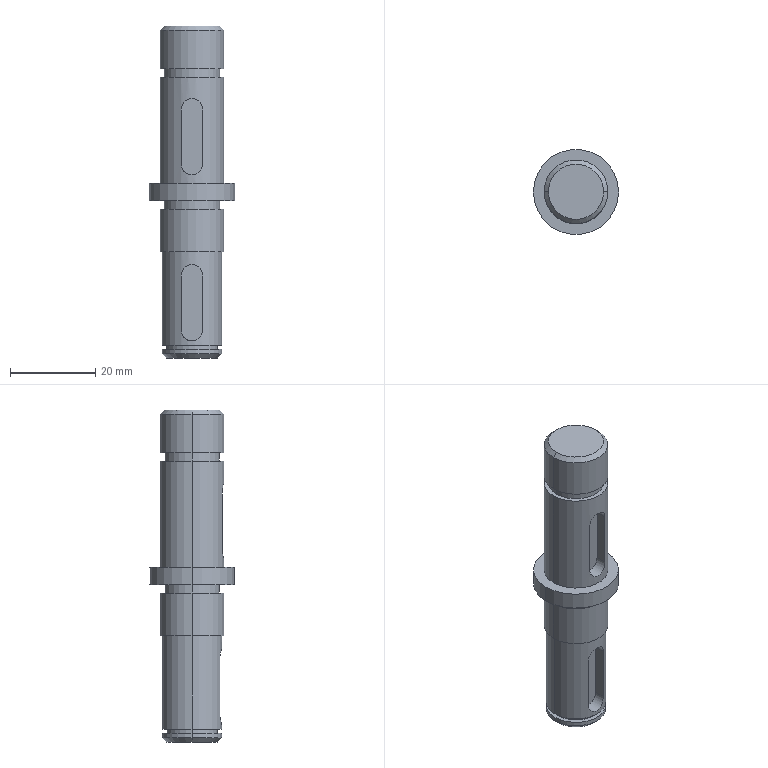Part | SolidWorks | features ICE 10, Chamfer 1, Extrusion 1 | 1 solid | 44 faces | box 20 x 20 x 78 mm | volume 13019 mm3 | cylinder 24 | plane 16 | cone 4 | commonest cylinder face diameters 5 x6 15 x6 13 x4 14 x4 12 x2 20 x2
STEP:
#1=CARTESIAN_POINT('',(0.,-7.5,61.));
#2=VERTEX_POINT('',#1);
#3=CARTESIAN_POINT('',(2.5,-7.071,58.5));
#4=VERTEX_POINT('',#3);
#5=CARTESIAN_POINT('',(0.,-7.5,61.));
#6=CARTESIAN_POINT('',(0.1643,-7.5,61.));
#7=CARTESIAN_POINT('',(0.3311,-7.494,60.983));
#8=CARTESIAN_POINT('',(0.6524,-7.473,60.919));
#9=CARTESIAN_POINT('',(0.8088,-7.458,60.871));
#10=CARTESIAN_POINT('',(1.113,-7.419,60.745));
#11=CARTESIAN_POINT('',(1.257,-7.395,60.667));
#12=CARTESIAN_POINT('',(1.526,-7.344,60.487));
#13=CARTESIAN_POINT('',(1.653,-7.316,60.382));
#14=CARTESIAN_POINT('',(1.883,-7.261,60.152));
#15=CARTESIAN_POINT('',(1.986,-7.233,60.027));
#16=CARTESIAN_POINT('',(2.167,-7.181,59.758));
#17=CARTESIAN_POINT('',(2.245,-7.156,59.612));
#18=CARTESIAN_POINT('',(2.37,-7.116,59.311));
#19=CARTESIAN_POINT('',(2.418,-7.1,59.156));
#20=CARTESIAN_POINT('',(2.483,-7.077,58.832));
#21=CARTESIAN_POINT('',(2.5,-7.071,58.666));
#22=CARTESIAN_POINT('',(2.5,-7.071,58.5));
#23=B_SPLINE_CURVE_WITH_KNOTS('',3,(#5,#6,#7,#8,#9,#10,#11,#12,#13,#14,#15,#16,#17,#18,#19,#20,#21,#22),.UNSPECIFIED.,.F.,.F.,(4,2,2,2,2,2,2,2,4),(0.003937,0.004429,0.004921,0.005412,0.005904,0.006395,0.006887,0.007378,0.00787),.UNSPECIFIED.);
#24=EDGE_CURVE('',#2,#4,#23,.T.);
#25=ORIENTED_EDGE('',*,*,#24,.F.);
#26=CARTESIAN_POINT('',(0.,-4.5,61.));
#27=VERTEX_POINT('',#26);
#28=CARTESIAN_POINT('',(0.,-14.5,61.));
#29=DIRECTION('',(0.,1.,0.));
#30=VECTOR('',#29,1000.);
#31=LINE('',#28,#30);
#32=EDGE_CURVE('',#2,#27,#31,.T.);
#33=ORIENTED_EDGE('',*,*,#32,.T.);
#34=CARTESIAN_POINT('',(2.5,-4.5,58.5));
#35=VERTEX_POINT('',#34);
#36=CARTESIAN_POINT('',(0.,-4.5,58.5));
#37=DIRECTION('',(0.,1.,0.));
#38=DIRECTION('',(0.,0.,1.));
#39=AXIS2_PLACEMENT_3D('',#36,#37,#38);
#40=CIRCLE('',#39,2.5);
#41=EDGE_CURVE('',#27,#35,#40,.T.);
#42=ORIENTED_EDGE('',*,*,#41,.T.);
#43=CARTESIAN_POINT('',(2.5,-14.5,58.5));
#44=DIRECTION('',(0.,1.,0.));
#45=VECTOR('',#44,1000.);
#46=LINE('',#43,#45);
#47=EDGE_CURVE('',#4,#35,#46,.T.);
#48=ORIENTED_EDGE('',*,*,#47,.F.);
#49=EDGE_LOOP('',(#25,#33,#42,#48));
#50=FACE_OUTER_BOUND('',#49,.T.);
#51=CARTESIAN_POINT('',(0.,-14.5,58.5));
#52=DIRECTION('',(0.,1.,0.));
#53=DIRECTION('',(0.,0.,1.));
#54=AXIS2_PLACEMENT_3D('',#51,#52,#53);
#55=CYLINDRICAL_SURFACE('',#54,2.5);
#56=ADVANCED_FACE('',(#50),#55,.F.);
#57=CARTESIAN_POINT('',(0.,-7.,22.));
#58=VERTEX_POINT('',#57);
#59=CARTESIAN_POINT('',(2.5,-6.538,19.5));
#60=VERTEX_POINT('',#59);
#61=CARTESIAN_POINT('',(0.,-7.,22.));
#62=CARTESIAN_POINT('',(0.1645,-7.,22.));
#63=CARTESIAN_POINT('',(0.3315,-6.994,21.983));
#64=CARTESIAN_POINT('',(0.653,-6.971,21.919));
#65=CARTESIAN_POINT('',(0.8095,-6.955,21.871));
#66=CARTESIAN_POINT('',(1.114,-6.913,21.744));
#67=CARTESIAN_POINT('',(1.257,-6.888,21.667));
#68=CARTESIAN_POINT('',(1.527,-6.833,21.486));
#69=CARTESIAN_POINT('',(1.654,-6.803,21.382));
#70=CARTESIAN_POINT('',(1.883,-6.743,21.152));
#71=CARTESIAN_POINT('',(1.986,-6.713,21.028));
#72=CARTESIAN_POINT('',(2.166,-6.657,20.758));
#73=CARTESIAN_POINT('',(2.245,-6.631,20.612));
#74=CARTESIAN_POINT('',(2.37,-6.587,20.312));
#75=CARTESIAN_POINT('',(2.418,-6.569,20.156));
#76=CARTESIAN_POINT('',(2.483,-6.545,19.833));
#77=CARTESIAN_POINT('',(2.5,-6.538,19.667));
#78=CARTESIAN_POINT('',(2.5,-6.538,19.5));
#79=B_SPLINE_CURVE_WITH_KNOTS('',3,(#61,#62,#63,#64,#65,#66,#67,#68,#69,#70,#71,#72,#73,#74,#75,#76,#77,#78),.UNSPECIFIED.,.F.,.F.,(4,2,2,2,2,2,2,2,4),(0.003942,0.004434,0.004926,0.005418,0.00591,0.006402,0.006894,0.007386,0.007878),.UNSPECIFIED.);
#80=EDGE_CURVE('',#58,#60,#79,.T.);
#81=ORIENTED_EDGE('',*,*,#80,.F.);
#82=CARTESIAN_POINT('',(0.,-4.,22.));
#83=VERTEX_POINT('',#82);
#84=CARTESIAN_POINT('',(0.,-14.,22.));
#85=DIRECTION('',(0.,1.,0.));
#86=VECTOR('',#85,1000.);
#87=LINE('',#84,#86);
#88=EDGE_CURVE('',#58,#83,#87,.T.);
#89=ORIENTED_EDGE('',*,*,#88,.T.);
#90=CARTESIAN_POINT('',(2.5,-4.,19.5));
#91=VERTEX_POINT('',#90);
#92=CARTESIAN_POINT('',(0.,-4.,19.5));
#93=DIRECTION('',(0.,1.,0.));
#94=DIRECTION('',(0.,0.,1.));
#95=AXIS2_PLACEMENT_3D('',#92,#93,#94);
#96=CIRCLE('',#95,2.5);
#97=EDGE_CURVE('',#83,#91,#96,.T.);
#98=ORIENTED_EDGE('',*,*,#97,.T.);
#99=CARTESIAN_POINT('',(2.5,-14.,19.5));
#100=DIRECTION('',(0.,1.,0.));
#101=VECTOR('',#100,1000.);
#102=LINE('',#99,#101);
#103=EDGE_CURVE('',#60,#91,#102,.T.);
#104=ORIENTED_EDGE('',*,*,#103,.F.);
#105=EDGE_LOOP('',(#81,#89,#98,#104));
#106=FACE_OUTER_BOUND('',#105,.T.);
#107=CARTESIAN_POINT('',(0.,-14.,19.5));
#108=DIRECTION('',(0.,1.,0.));
#109=DIRECTION('',(0.,0.,1.));
#110=AXIS2_PLACEMENT_3D('',#107,#108,#109);
#111=CYLINDRICAL_SURFACE('',#110,2.5);
#112=ADVANCED_FACE('',(#106),#111,.F.);
#113=CARTESIAN_POINT('',(6.5,0.,78.));
#114=VERTEX_POINT('',#113);
#115=CARTESIAN_POINT('',(-6.5,0.,78.));
#116=VERTEX_POINT('',#115);
#117=CARTESIAN_POINT('',(0.,0.,78.));
#118=DIRECTION('',(0.,0.,1.));
#119=DIRECTION('',(1.,0.,0.));
#120=AXIS2_PLACEMENT_3D('',#117,#118,#119);
#121=CIRCLE('',#120,6.5);
#122=EDGE_CURVE('',#114,#116,#121,.T.);
#123=ORIENTED_EDGE('',*,*,#122,.F.);
#124=CARTESIAN_POINT('',(7.5,0.,77.));
#125=VERTEX_POINT('',#124);
#126=CARTESIAN_POINT('',(6.5,0.,78.));
#127=DIRECTION('',(0.7071,0.,-0.7071));
#128=VECTOR('',#127,1000.);
#129=LINE('',#126,#128);
#130=EDGE_CURVE('',#114,#125,#129,.T.);
#131=ORIENTED_EDGE('',*,*,#130,.T.);
#132=CARTESIAN_POINT('',(-7.5,0.,77.));
#133=VERTEX_POINT('',#132);
#134=CARTESIAN_POINT('',(0.,0.,77.));
#135=DIRECTION('',(0.,0.,-1.));
#136=DIRECTION('',(1.,0.,0.));
#137=AXIS2_PLACEMENT_3D('',#134,#135,#136);
#138=CIRCLE('',#137,7.5);
#139=EDGE_CURVE('',#133,#125,#138,.T.);
#140=ORIENTED_EDGE('',*,*,#139,.F.);
#141=CARTESIAN_POINT('',(-6.5,0.,78.));
#142=DIRECTION('',(-0.7071,0.,-0.7071));
#143=VECTOR('',#142,1000.);
#144=LINE('',#141,#143);
#145=EDGE_CURVE('',#116,#133,#144,.T.);
#146=ORIENTED_EDGE('',*,*,#145,.F.);
#147=EDGE_LOOP('',(#123,#131,#140,#146));
#148=FACE_OUTER_BOUND('',#147,.T.);
#149=CARTESIAN_POINT('',(0.,0.,78.));
#150=DIRECTION('',(0.,0.,-1.));
#151=DIRECTION('',(-1.,0.,0.));
#152=AXIS2_PLACEMENT_3D('',#149,#150,#151);
#153=CONICAL_SURFACE('',#152,6.5,0.7854);
#154=ADVANCED_FACE('',(#148),#153,.T.);
#155=CARTESIAN_POINT('',(-6.,0.,0.));
#156=VERTEX_POINT('',#155);
#157=CARTESIAN_POINT('',(6.,0.,0.));
#158=VERTEX_POINT('',#157);
#159=CARTESIAN_POINT('',(0.,0.,0.));
#160=DIRECTION('',(0.,0.,-1.));
#161=DIRECTION('',(1.,0.,0.));
#162=AXIS2_PLACEMENT_3D('',#159,#160,#161);
#163=CIRCLE('',#162,6.);
#164=EDGE_CURVE('',#156,#158,#163,.T.);
#165=ORIENTED_EDGE('',*,*,#164,.F.);
#166=CARTESIAN_POINT('',(-7.,0.,1.));
#167=VERTEX_POINT('',#166);
#168=CARTESIAN_POINT('',(-7.,0.,1.));
#169=DIRECTION('',(-0.7071,0.,0.7071));
#170=VECTOR('',#169,1000.);
#171=LINE('',#168,#170);
#172=EDGE_CURVE('',#156,#167,#171,.T.);
#173=ORIENTED_EDGE('',*,*,#172,.T.);
#174=CARTESIAN_POINT('',(7.,0.,1.));
#175=VERTEX_POINT('',#174);
#176=CARTESIAN_POINT('',(0.,0.,1.));
#177=DIRECTION('',(0.,0.,1.));
#178=DIRECTION('',(1.,0.,0.));
#179=AXIS2_PLACEMENT_3D('',#176,#177,#178);
#180=CIRCLE('',#179,7.);
#181=EDGE_CURVE('',#175,#167,#180,.T.);
#182=ORIENTED_EDGE('',*,*,#181,.F.);
#183=CARTESIAN_POINT('',(7.,0.,1.));
#184=DIRECTION('',(0.7071,0.,0.7071));
#185=VECTOR('',#184,1000.);
#186=LINE('',#183,#185);
#187=EDGE_CURVE('',#158,#175,#186,.T.);
#188=ORIENTED_EDGE('',*,*,#187,.F.);
#189=EDGE_LOOP('',(#165,#173,#182,#188));
#190=FACE_OUTER_BOUND('',#189,.T.);
#191=CARTESIAN_POINT('',(0.,0.,1.));
#192=DIRECTION('',(0.,0.,1.));
#193=DIRECTION('',(1.,0.,0.));
#194=AXIS2_PLACEMENT_3D('',#191,#192,#193);
#195=CONICAL_SURFACE('',#194,7.,0.7854);
#196=ADVANCED_FACE('',(#190),#195,.T.);
#197=ORIENTED_EDGE('',*,*,#139,.T.);
#198=CARTESIAN_POINT('',(7.5,0.,68.));
#199=VERTEX_POINT('',#198);
#200=CARTESIAN_POINT('',(7.5,0.,78.));
#201=DIRECTION('',(0.,0.,-1.));
#202=VECTOR('',#201,1000.);
#203=LINE('',#200,#202);
#204=EDGE_CURVE('',#125,#199,#203,.T.);
#205=ORIENTED_EDGE('',*,*,#204,.T.);
#206=CARTESIAN_POINT('',(-7.5,0.,68.));
#207=VERTEX_POINT('',#206);
#208=CARTESIAN_POINT('',(0.,0.,68.));
#209=DIRECTION('',(0.,0.,1.));
#210=DIRECTION('',(1.,0.,0.));
#211=AXIS2_PLACEMENT_3D('',#208,#209,#210);
#212=CIRCLE('',#211,7.5);
#213=EDGE_CURVE('',#199,#207,#212,.T.);
#214=ORIENTED_EDGE('',*,*,#213,.T.);
#215=CARTESIAN_POINT('',(-7.5,0.,78.));
#216=DIRECTION('',(0.,0.,-1.));
#217=VECTOR('',#216,1000.);
#218=LINE('',#215,#217);
#219=EDGE_CURVE('',#133,#207,#218,.T.);
#220=ORIENTED_EDGE('',*,*,#219,.F.);
#221=EDGE_LOOP('',(#197,#205,#214,#220));
#222=FACE_OUTER_BOUND('',#221,.T.);
#223=CARTESIAN_POINT('',(0.,0.,78.));
#224=DIRECTION('',(0.,0.,-1.));
#225=DIRECTION('',(-1.,0.,0.));
#226=AXIS2_PLACEMENT_3D('',#223,#224,#225);
#227=CYLINDRICAL_SURFACE('',#226,7.5);
#228=ADVANCED_FACE('',(#222),#227,.T.);
#229=CARTESIAN_POINT('',(6.5,0.,68.));
#230=VERTEX_POINT('',#229);
#231=CARTESIAN_POINT('',(-6.5,0.,68.));
#232=VERTEX_POINT('',#231);
#233=CARTESIAN_POINT('',(0.,0.,68.));
#234=DIRECTION('',(0.,0.,1.));
#235=DIRECTION('',(1.,0.,0.));
#236=AXIS2_PLACEMENT_3D('',#233,#234,#235);
#237=CIRCLE('',#236,6.5);
#238=EDGE_CURVE('',#230,#232,#237,.T.);
#239=ORIENTED_EDGE('',*,*,#238,.F.);
#240=CARTESIAN_POINT('',(6.5,0.,66.));
#241=VERTEX_POINT('',#240);
#242=CARTESIAN_POINT('',(6.5,0.,68.));
#243=DIRECTION('',(0.,0.,-1.));
#244=VECTOR('',#243,1000.);
#245=LINE('',#242,#244);
#246=EDGE_CURVE('',#230,#241,#245,.T.);
#247=ORIENTED_EDGE('',*,*,#246,.T.);
#248=CARTESIAN_POINT('',(-6.5,0.,66.));
#249=VERTEX_POINT('',#248);
#250=CARTESIAN_POINT('',(0.,0.,66.));
#251=DIRECTION('',(0.,0.,1.));
#252=DIRECTION('',(1.,0.,0.));
#253=AXIS2_PLACEMENT_3D('',#250,#251,#252);
#254=CIRCLE('',#253,6.5);
#255=EDGE_CURVE('',#241,#249,#254,.T.);
#256=ORIENTED_EDGE('',*,*,#255,.T.);
#257=CARTESIAN_POINT('',(-6.5,0.,68.));
#258=DIRECTION('',(0.,0.,-1.));
#259=VECTOR('',#258,1000.);
#260=LINE('',#257,#259);
#261=EDGE_CURVE('',#232,#249,#260,.T.);
#262=ORIENTED_EDGE('',*,*,#261,.F.);
#263=EDGE_LOOP('',(#239,#247,#256,#262));
#264=FACE_OUTER_BOUND('',#263,.T.);
#265=CARTESIAN_POINT('',(0.,0.,68.));
#266=DIRECTION('',(0.,0.,-1.));
#267=DIRECTION('',(-1.,0.,0.));
#268=AXIS2_PLACEMENT_3D('',#265,#266,#267);
#269=CYLINDRICAL_SURFACE('',#268,6.5);
#270=ADVANCED_FACE('',(#264),#269,.T.);
#271=CARTESIAN_POINT('',(7.5,0.,66.));
#272=VERTEX_POINT('',#271);
#273=CARTESIAN_POINT('',(-7.5,0.,66.));
#274=VERTEX_POINT('',#273);
#275=CARTESIAN_POINT('',(0.,0.,66.));
#276=DIRECTION('',(0.,0.,1.));
#277=DIRECTION('',(1.,0.,0.));
#278=AXIS2_PLACEMENT_3D('',#275,#276,#277);
#279=CIRCLE('',#278,7.5);
#280=EDGE_CURVE('',#272,#274,#279,.T.);
#281=ORIENTED_EDGE('',*,*,#280,.F.);
#282=CARTESIAN_POINT('',(7.5,0.,41.));
#283=VERTEX_POINT('',#282);
#284=CARTESIAN_POINT('',(7.5,0.,66.));
#285=DIRECTION('',(0.,0.,-1.));
#286=VECTOR('',#285,1000.);
#287=LINE('',#284,#286);
#288=EDGE_CURVE('',#272,#283,#287,.T.);
#289=ORIENTED_EDGE('',*,*,#288,.T.);
#290=CARTESIAN_POINT('',(-7.5,0.,41.));
#291=VERTEX_POINT('',#290);
#292=CARTESIAN_POINT('',(0.,0.,41.));
#293=DIRECTION('',(0.,0.,1.));
#294=DIRECTION('',(1.,0.,0.));
#295=AXIS2_PLACEMENT_3D('',#292,#293,#294);
#296=CIRCLE('',#295,7.5);
#297=EDGE_CURVE('',#283,#291,#296,.T.);
#298=ORIENTED_EDGE('',*,*,#297,.T.);
#299=CARTESIAN_POINT('',(-7.5,0.,66.));
#300=DIRECTION('',(0.,0.,-1.));
#301=VECTOR('',#300,1000.);
#302=LINE('',#299,#301);
#303=EDGE_CURVE('',#274,#291,#302,.T.);
#304=ORIENTED_EDGE('',*,*,#303,.F.);
#305=EDGE_LOOP('',(#281,#289,#298,#304));
#306=FACE_OUTER_BOUND('',#305,.T.);
#307=CARTESIAN_POINT('',(0.,0.,66.));
#308=DIRECTION('',(0.,0.,-1.));
#309=DIRECTION('',(-1.,0.,0.));
#310=AXIS2_PLACEMENT_3D('',#307,#308,#309);
#311=CYLINDRICAL_SURFACE('',#310,7.5);
#312=ADVANCED_FACE('',(#306),#311,.T.);
#313=CARTESIAN_POINT('',(10.,0.,41.));
#314=VERTEX_POINT('',#313);
#315=CARTESIAN_POINT('',(-10.,0.,41.));
#316=VERTEX_POINT('',#315);
#317=CARTESIAN_POINT('',(0.,0.,41.));
#318=DIRECTION('',(0.,0.,1.));
#319=DIRECTION('',(1.,0.,0.));
#320=AXIS2_PLACEMENT_3D('',#317,#318,#319);
#321=CIRCLE('',#320,10.);
#322=EDGE_CURVE('',#314,#316,#321,.T.);
#323=ORIENTED_EDGE('',*,*,#322,.F.);
#324=CARTESIAN_POINT('',(10.,0.,37.));
#325=VERTEX_POINT('',#324);
#326=CARTESIAN_POINT('',(10.,0.,41.));
#327=DIRECTION('',(0.,0.,-1.));
#328=VECTOR('',#327,1000.);
#329=LINE('',#326,#328);
#330=EDGE_CURVE('',#314,#325,#329,.T.);
#331=ORIENTED_EDGE('',*,*,#330,.T.);
#332=CARTESIAN_POINT('',(-10.,0.,37.));
#333=VERTEX_POINT('',#332);
#334=CARTESIAN_POINT('',(0.,0.,37.));
#335=DIRECTION('',(0.,0.,1.));
#336=DIRECTION('',(1.,0.,0.));
#337=AXIS2_PLACEMENT_3D('',#334,#335,#336);
#338=CIRCLE('',#337,10.);
#339=EDGE_CURVE('',#325,#333,#338,.T.);
#340=ORIENTED_EDGE('',*,*,#339,.T.);
#341=CARTESIAN_POINT('',(-10.,0.,41.));
#342=DIRECTION('',(0.,0.,-1.));
#343=VECTOR('',#342,1000.);
#344=LINE('',#341,#343);
#345=EDGE_CURVE('',#316,#333,#344,.T.);
#346=ORIENTED_EDGE('',*,*,#345,.F.);
#347=EDGE_LOOP('',(#323,#331,#340,#346));
#348=FACE_OUTER_BOUND('',#347,.T.);
#349=CARTESIAN_POINT('',(0.,0.,41.));
#350=DIRECTION('',(0.,0.,-1.));
#351=DIRECTION('',(-1.,0.,0.));
#352=AXIS2_PLACEMENT_3D('',#349,#350,#351);
#353=CYLINDRICAL_SURFACE('',#352,10.);
#354=ADVANCED_FACE('',(#348),#353,.T.);
#355=CARTESIAN_POINT('',(6.5,0.,37.));
#356=VERTEX_POINT('',#355);
#357=CARTESIAN_POINT('',(-6.5,0.,37.));
#358=VERTEX_POINT('',#357);
#359=CARTESIAN_POINT('',(0.,0.,37.));
#360=DIRECTION('',(0.,0.,1.));
#361=DIRECTION('',(1.,0.,0.));
#362=AXIS2_PLACEMENT_3D('',#359,#360,#361);
#363=CIRCLE('',#362,6.5);
#364=EDGE_CURVE('',#356,#358,#363,.T.);
#365=ORIENTED_EDGE('',*,*,#364,.F.);
#366=CARTESIAN_POINT('',(6.5,0.,35.));
#367=VERTEX_POINT('',#366);
#368=CARTESIAN_POINT('',(6.5,0.,37.));
#369=DIRECTION('',(0.,0.,-1.));
#370=VECTOR('',#369,1000.);
#371=LINE('',#368,#370);
#372=EDGE_CURVE('',#356,#367,#371,.T.);
#373=ORIENTED_EDGE('',*,*,#372,.T.);
#374=CARTESIAN_POINT('',(-6.5,0.,35.));
#375=VERTEX_POINT('',#374);
#376=CARTESIAN_POINT('',(0.,0.,35.));
#377=DIRECTION('',(0.,0.,1.));
#378=DIRECTION('',(1.,0.,0.));
#379=AXIS2_PLACEMENT_3D('',#376,#377,#378);
#380=CIRCLE('',#379,6.5);
#381=EDGE_CURVE('',#367,#375,#380,.T.);
#382=ORIENTED_EDGE('',*,*,#381,.T.);
#383=CARTESIAN_POINT('',(-6.5,0.,37.));
#384=DIRECTION('',(0.,0.,-1.));
#385=VECTOR('',#384,1000.);
#386=LINE('',#383,#385);
#387=EDGE_CURVE('',#358,#375,#386,.T.);
#388=ORIENTED_EDGE('',*,*,#387,.F.);
#389=EDGE_LOOP('',(#365,#373,#382,#388));
#390=FACE_OUTER_BOUND('',#389,.T.);
#391=CARTESIAN_POINT('',(0.,0.,37.));
#392=DIRECTION('',(0.,0.,-1.));
#393=DIRECTION('',(-1.,0.,0.));
#394=AXIS2_PLACEMENT_3D('',#391,#392,#393);
#395=CYLINDRICAL_SURFACE('',#394,6.5);
#396=ADVANCED_FACE('',(#390),#395,.T.);
#397=CARTESIAN_POINT('',(7.5,0.,35.));
#398=VERTEX_POINT('',#397);
#399=CARTESIAN_POINT('',(-7.5,0.,35.));
#400=VERTEX_POINT('',#399);
#401=CARTESIAN_POINT('',(0.,0.,35.));
#402=DIRECTION('',(0.,0.,1.));
#403=DIRECTION('',(1.,0.,0.));
#404=AXIS2_PLACEMENT_3D('',#401,#402,#403);
#405=CIRCLE('',#404,7.5);
#406=EDGE_CURVE('',#398,#400,#405,.T.);
#407=ORIENTED_EDGE('',*,*,#406,.F.);
#408=CARTESIAN_POINT('',(7.5,0.,25.));
#409=VERTEX_POINT('',#408);
#410=CARTESIAN_POINT('',(7.5,0.,35.));
#411=DIRECTION('',(0.,0.,-1.));
#412=VECTOR('',#411,1000.);
#413=LINE('',#410,#412);
#414=EDGE_CURVE('',#398,#409,#413,.T.);
#415=ORIENTED_EDGE('',*,*,#414,.T.);
#416=CARTESIAN_POINT('',(-7.5,0.,25.));
#417=VERTEX_POINT('',#416);
#418=CARTESIAN_POINT('',(0.,0.,25.));
#419=DIRECTION('',(0.,0.,1.));
#420=DIRECTION('',(1.,0.,0.));
#421=AXIS2_PLACEMENT_3D('',#418,#419,#420);
#422=CIRCLE('',#421,7.5);
#423=EDGE_CURVE('',#409,#417,#422,.T.);
#424=ORIENTED_EDGE('',*,*,#423,.T.);
#425=CARTESIAN_POINT('',(-7.5,0.,35.));
#426=DIRECTION('',(0.,0.,-1.));
#427=VECTOR('',#426,1000.);
#428=LINE('',#425,#427);
#429=EDGE_CURVE('',#400,#417,#428,.T.);
#430=ORIENTED_EDGE('',*,*,#429,.F.);
#431=EDGE_LOOP('',(#407,#415,#424,#430));
#432=FACE_OUTER_BOUND('',#431,.T.);
#433=CARTESIAN_POINT('',(0.,0.,35.));
#434=DIRECTION('',(0.,0.,-1.));
#435=DIRECTION('',(-1.,0.,0.));
#436=AXIS2_PLACEMENT_3D('',#433,#434,#435);
#437=CYLINDRICAL_SURFACE('',#436,7.5);
#438=ADVANCED_FACE('',(#432),#437,.T.);
#439=CARTESIAN_POINT('',(7.,0.,25.));
#440=VERTEX_POINT('',#439);
#441=CARTESIAN_POINT('',(-7.,0.,25.));
#442=VERTEX_POINT('',#441);
#443=CARTESIAN_POINT('',(0.,0.,25.));
#444=DIRECTION('',(0.,0.,1.));
#445=DIRECTION('',(1.,0.,0.));
#446=AXIS2_PLACEMENT_3D('',#443,#444,#445);
#447=CIRCLE('',#446,7.);
#448=EDGE_CURVE('',#440,#442,#447,.T.);
#449=ORIENTED_EDGE('',*,*,#448,.F.);
#450=CARTESIAN_POINT('',(7.,0.,3.));
#451=VERTEX_POINT('',#450);
#452=CARTESIAN_POINT('',(7.,0.,25.));
#453=DIRECTION('',(0.,0.,-1.));
#454=VECTOR('',#453,1000.);
#455=LINE('',#452,#454);
#456=EDGE_CURVE('',#440,#451,#455,.T.);
#457=ORIENTED_EDGE('',*,*,#456,.T.);
#458=CARTESIAN_POINT('',(-7.,0.,3.));
#459=VERTEX_POINT('',#458);
#460=CARTESIAN_POINT('',(0.,0.,3.));
#461=DIRECTION('',(0.,0.,1.));
#462=DIRECTION('',(1.,0.,0.));
#463=AXIS2_PLACEMENT_3D('',#460,#461,#462);
#464=CIRCLE('',#463,7.);
#465=EDGE_CURVE('',#451,#459,#464,.T.);
#466=ORIENTED_EDGE('',*,*,#465,.T.);
#467=CARTESIAN_POINT('',(-7.,0.,25.));
#468=DIRECTION('',(0.,0.,-1.));
#469=VECTOR('',#468,1000.);
#470=LINE('',#467,#469);
#471=EDGE_CURVE('',#442,#459,#470,.T.);
#472=ORIENTED_EDGE('',*,*,#471,.F.);
#473=EDGE_LOOP('',(#449,#457,#466,#472));
#474=FACE_OUTER_BOUND('',#473,.T.);
#475=CARTESIAN_POINT('',(0.,0.,25.));
#476=DIRECTION('',(0.,0.,-1.));
#477=DIRECTION('',(-1.,0.,0.));
#478=AXIS2_PLACEMENT_3D('',#475,#476,#477);
#479=CYLINDRICAL_SURFACE('',#478,7.);
#480=ADVANCED_FACE('',(#474),#479,.T.);
#481=CARTESIAN_POINT('',(6.,0.,3.));
#482=VERTEX_POINT('',#481);
#483=CARTESIAN_POINT('',(-6.,0.,3.));
#484=VERTEX_POINT('',#483);
#485=CARTESIAN_POINT('',(0.,0.,3.));
#486=DIRECTION('',(0.,0.,1.));
#487=DIRECTION('',(1.,0.,0.));
#488=AXIS2_PLACEMENT_3D('',#485,#486,#487);
#489=CIRCLE('',#488,6.);
#490=EDGE_CURVE('',#482,#484,#489,.T.);
#491=ORIENTED_EDGE('',*,*,#490,.F.);
#492=CARTESIAN_POINT('',(6.,0.,2.));
#493=VERTEX_POINT('',#492);
#494=CARTESIAN_POINT('',(6.,0.,3.));
#495=DIRECTION('',(0.,0.,-1.));
#496=VECTOR('',#495,1000.);
#497=LINE('',#494,#496);
#498=EDGE_CURVE('',#482,#493,#497,.T.);
#499=ORIENTED_EDGE('',*,*,#498,.T.);
#500=CARTESIAN_POINT('',(-6.,0.,2.));
#501=VERTEX_POINT('',#500);
#502=CARTESIAN_POINT('',(0.,0.,2.));
#503=DIRECTION('',(0.,0.,1.));
#504=DIRECTION('',(1.,0.,0.));
#505=AXIS2_PLACEMENT_3D('',#502,#503,#504);
#506=CIRCLE('',#505,6.);
#507=EDGE_CURVE('',#493,#501,#506,.T.);
#508=ORIENTED_EDGE('',*,*,#507,.T.);
#509=CARTESIAN_POINT('',(-6.,0.,3.));
#510=DIRECTION('',(0.,0.,-1.));
#511=VECTOR('',#510,1000.);
#512=LINE('',#509,#511);
#513=EDGE_CURVE('',#484,#501,#512,.T.);
#514=ORIENTED_EDGE('',*,*,#513,.F.);
#515=EDGE_LOOP('',(#491,#499,#508,#514));
#516=FACE_OUTER_BOUND('',#515,.T.);
#517=CARTESIAN_POINT('',(0.,0.,3.));
#518=DIRECTION('',(0.,0.,-1.));
#519=DIRECTION('',(-1.,0.,0.));
#520=AXIS2_PLACEMENT_3D('',#517,#518,#519);
#521=CYLINDRICAL_SURFACE('',#520,6.);
#522=ADVANCED_FACE('',(#516),#521,.T.);
#523=CARTESIAN_POINT('',(7.,0.,2.));
#524=VERTEX_POINT('',#523);
#525=CARTESIAN_POINT('',(-7.,0.,2.));
#526=VERTEX_POINT('',#525);
#527=CARTESIAN_POINT('',(0.,0.,2.));
#528=DIRECTION('',(0.,0.,1.));
#529=DIRECTION('',(1.,0.,0.));
#530=AXIS2_PLACEMENT_3D('',#527,#528,#529);
#531=CIRCLE('',#530,7.);
#532=EDGE_CURVE('',#524,#526,#531,.T.);
#533=ORIENTED_EDGE('',*,*,#532,.F.);
#534=CARTESIAN_POINT('',(7.,0.,2.));
#535=DIRECTION('',(0.,0.,-1.));
#536=VECTOR('',#535,1000.);
#537=LINE('',#534,#536);
#538=EDGE_CURVE('',#524,#175,#537,.T.);
#539=ORIENTED_EDGE('',*,*,#538,.T.);
#540=ORIENTED_EDGE('',*,*,#181,.T.);
#541=CARTESIAN_POINT('',(-7.,0.,2.));
#542=DIRECTION('',(0.,0.,-1.));
#543=VECTOR('',#542,1000.);
#544=LINE('',#541,#543);
#545=EDGE_CURVE('',#526,#167,#544,.T.);
#546=ORIENTED_EDGE('',*,*,#545,.F.);
#547=EDGE_LOOP('',(#533,#539,#540,#546));
#548=FACE_OUTER_BOUND('',#547,.T.);
#549=CARTESIAN_POINT('',(0.,0.,2.));
#550=DIRECTION('',(0.,0.,-1.));
#551=DIRECTION('',(-1.,0.,0.));
#552=AXIS2_PLACEMENT_3D('',#549,#550,#551);
#553=CYLINDRICAL_SURFACE('',#552,7.);
#554=ADVANCED_FACE('',(#548),#553,.T.);
#555=ORIENTED_EDGE('',*,*,#538,.F.);
#556=CARTESIAN_POINT('',(0.,0.,2.));
#557=DIRECTION('',(0.,0.,1.));
#558=DIRECTION('',(1.,0.,0.));
#559=AXIS2_PLACEMENT_3D('',#556,#557,#558);
#560=CIRCLE('',#559,7.);
#561=EDGE_CURVE('',#526,#524,#560,.T.);
#562=ORIENTED_EDGE('',*,*,#561,.F.);
#563=ORIENTED_EDGE('',*,*,#545,.T.);
#564=CARTESIAN_POINT('',(0.,0.,1.));
#565=DIRECTION('',(0.,0.,1.));
#566=DIRECTION('',(1.,0.,0.));
#567=AXIS2_PLACEMENT_3D('',#564,#565,#566);
#568=CIRCLE('',#567,7.);
#569=EDGE_CURVE('',#167,#175,#568,.T.);
#570=ORIENTED_EDGE('',*,*,#569,.T.);
#571=EDGE_LOOP('',(#555,#562,#563,#570));
#572=FACE_OUTER_BOUND('',#571,.T.);
#573=CARTESIAN_POINT('',(0.,0.,2.));
#574=DIRECTION('',(0.,0.,-1.));
#575=DIRECTION('',(-1.,0.,0.));
#576=AXIS2_PLACEMENT_3D('',#573,#574,#575);
#577=CYLINDRICAL_SURFACE('',#576,7.);
#578=ADVANCED_FACE('',(#572),#577,.T.);
#579=CARTESIAN_POINT('',(0.,0.,2.));
#580=DIRECTION('',(0.,0.,1.));
#581=DIRECTION('',(1.,0.,0.));
#582=AXIS2_PLACEMENT_3D('',#579,#580,#581);
#583=CIRCLE('',#582,6.);
#584=EDGE_CURVE('',#501,#493,#583,.T.);
#585=ORIENTED_EDGE('',*,*,#584,.F.);
#586=ORIENTED_EDGE('',*,*,#507,.F.);
#587=EDGE_LOOP('',(#585,#586));
#588=FACE_BOUND('',#587,.T.);
#589=ORIENTED_EDGE('',*,*,#561,.T.);
#590=ORIENTED_EDGE('',*,*,#532,.T.);
#591=EDGE_LOOP('',(#589,#590));
#592=FACE_OUTER_BOUND('',#591,.T.);
#593=CARTESIAN_POINT('',(0.,0.,2.));
#594=DIRECTION('',(0.,0.,1.));
#595=DIRECTION('',(1.,0.,0.));
#596=AXIS2_PLACEMENT_3D('',#593,#594,#595);
#597=PLANE('',#596);
#598=ADVANCED_FACE('',(#588,#592),#597,.T.);
#599=CARTESIAN_POINT('',(0.,0.,0.));
#600=DIRECTION('',(0.,0.,-1.));
#601=DIRECTION('',(1.,0.,0.));
#602=AXIS2_PLACEMENT_3D('',#599,#600,#601);
#603=CIRCLE('',#602,6.);
#604=EDGE_CURVE('',#158,#156,#603,.T.);
#605=ORIENTED_EDGE('',*,*,#604,.T.);
#606=ORIENTED_EDGE('',*,*,#164,.T.);
#607=EDGE_LOOP('',(#605,#606));
#608=FACE_OUTER_BOUND('',#607,.T.);
#609=CARTESIAN_POINT('',(0.,0.,0.));
#610=DIRECTION('',(0.,0.,1.));
#611=DIRECTION('',(1.,0.,0.));
#612=AXIS2_PLACEMENT_3D('',#609,#610,#611);
#613=PLANE('',#612);
#614=ADVANCED_FACE('',(#608),#613,.F.);
#615=ORIENTED_EDGE('',*,*,#498,.F.);
#616=CARTESIAN_POINT('',(0.,0.,3.));
#617=DIRECTION('',(0.,0.,1.));
#618=DIRECTION('',(1.,0.,0.));
#619=AXIS2_PLACEMENT_3D('',#616,#617,#618);
#620=CIRCLE('',#619,6.);
#621=EDGE_CURVE('',#484,#482,#620,.T.);
#622=ORIENTED_EDGE('',*,*,#621,.F.);
#623=ORIENTED_EDGE('',*,*,#513,.T.);
#624=ORIENTED_EDGE('',*,*,#584,.T.);
#625=EDGE_LOOP('',(#615,#622,#623,#624));
#626=FACE_OUTER_BOUND('',#625,.T.);
#627=CARTESIAN_POINT('',(0.,0.,3.));
#628=DIRECTION('',(0.,0.,-1.));
#629=DIRECTION('',(-1.,0.,0.));
#630=AXIS2_PLACEMENT_3D('',#627,#628,#629);
#631=CYLINDRICAL_SURFACE('',#630,6.);
#632=ADVANCED_FACE('',(#626),#631,.T.);
#633=ORIENTED_EDGE('',*,*,#456,.F.);
#634=CARTESIAN_POINT('',(0.,0.,25.));
#635=DIRECTION('',(0.,0.,1.));
#636=DIRECTION('',(1.,0.,0.));
#637=AXIS2_PLACEMENT_3D('',#634,#635,#636);
#638=CIRCLE('',#637,7.);
#639=EDGE_CURVE('',#442,#440,#638,.T.);
#640=ORIENTED_EDGE('',*,*,#639,.F.);
#641=ORIENTED_EDGE('',*,*,#471,.T.);
#642=CARTESIAN_POINT('',(0.,0.,3.));
#643=DIRECTION('',(0.,0.,1.));
#644=DIRECTION('',(1.,0.,0.));
#645=AXIS2_PLACEMENT_3D('',#642,#643,#644);
#646=CIRCLE('',#645,7.);
#647=EDGE_CURVE('',#459,#451,#646,.T.);
#648=ORIENTED_EDGE('',*,*,#647,.T.);
#649=EDGE_LOOP('',(#633,#640,#641,#648));
#650=FACE_OUTER_BOUND('',#649,.T.);
#651=CARTESIAN_POINT('',(2.5,-6.538,6.5));
#652=VERTEX_POINT('',#651);
#653=CARTESIAN_POINT('',(2.5,-6.538,25.));
#654=DIRECTION('',(0.,0.,1.));
#655=VECTOR('',#654,1000.);
#656=LINE('',#653,#655);
#657=EDGE_CURVE('',#652,#60,#656,.T.);
#658=ORIENTED_EDGE('',*,*,#657,.F.);
#659=CARTESIAN_POINT('',(-2.5,-6.538,6.5));
#660=VERTEX_POINT('',#659);
#661=CARTESIAN_POINT('',(2.5,-6.538,6.5));
#662=CARTESIAN_POINT('',(2.5,-6.538,6.333));
#663=CARTESIAN_POINT('',(2.484,-6.545,6.17));
#664=CARTESIAN_POINT('',(2.419,-6.569,5.849));
#665=CARTESIAN_POINT('',(2.371,-6.587,5.689));
#666=CARTESIAN_POINT('',(2.245,-6.631,5.387));
#667=CARTESIAN_POINT('',(2.168,-6.657,5.244));
#668=CARTESIAN_POINT('',(1.987,-6.713,4.974));
#669=CARTESIAN_POINT('',(1.882,-6.743,4.847));
#670=CARTESIAN_POINT('',(1.54,-6.833,4.504));
#671=CARTESIAN_POINT('',(1.263,-6.892,4.318));
#672=CARTESIAN_POINT('',(0.8128,-6.954,4.13));
#673=CARTESIAN_POINT('',(0.6538,-6.971,4.081));
#674=CARTESIAN_POINT('',(0.3305,-6.994,4.016));
#675=CARTESIAN_POINT('',(0.1674,-7.,4.));
#676=CARTESIAN_POINT('',(-0.1618,-7.,4.));
#677=CARTESIAN_POINT('',(-0.3289,-6.994,4.016));
#678=CARTESIAN_POINT('',(-0.6508,-6.972,4.081));
#679=CARTESIAN_POINT('',(-0.8074,-6.955,4.128));
#680=CARTESIAN_POINT('',(-1.112,-6.913,4.255));
#681=CARTESIAN_POINT('',(-1.256,-6.888,4.332));
#682=CARTESIAN_POINT('',(-1.525,-6.833,4.513));
#683=CARTESIAN_POINT('',(-1.653,-6.803,4.617));
#684=CARTESIAN_POINT('',(-1.882,-6.743,4.847));
#685=CARTESIAN_POINT('',(-1.985,-6.713,4.971));
#686=CARTESIAN_POINT('',(-2.166,-6.657,5.241));
#687=CARTESIAN_POINT('',(-2.244,-6.631,5.387));
#688=CARTESIAN_POINT('',(-2.37,-6.587,5.687));
#689=CARTESIAN_POINT('',(-2.418,-6.569,5.843));
#690=CARTESIAN_POINT('',(-2.483,-6.545,6.167));
#691=CARTESIAN_POINT('',(-2.5,-6.538,6.333));
#692=CARTESIAN_POINT('',(-2.5,-6.538,6.5));
#693=B_SPLINE_CURVE_WITH_KNOTS('',3,(#661,#662,#663,#664,#665,#666,#667,#668,#669,#670,#671,#672,#673,#674,#675,#676,#677,#678,#679,#680,#681,#682,#683,#684,#685,#686,#687,#688,#689,#690,#691,#692),.UNSPECIFIED.,.F.,.F.,(4,2,2,2,2,2,2,2,2,2,2,2,2,2,2,4),(0.,0.0004924,0.0009848,0.001477,0.00197,0.002954,0.003447,0.003939,0.004432,0.004924,0.005416,0.005909,0.006401,0.006894,0.007386,0.007878),.UNSPECIFIED.);
#694=EDGE_CURVE('',#652,#660,#693,.T.);
#695=ORIENTED_EDGE('',*,*,#694,.T.);
#696=CARTESIAN_POINT('',(-2.5,-6.538,19.5));
#697=VERTEX_POINT('',#696);
#698=CARTESIAN_POINT('',(-2.5,-6.538,25.));
#699=DIRECTION('',(0.,0.,1.));
#700=VECTOR('',#699,1000.);
#701=LINE('',#698,#700);
#702=EDGE_CURVE('',#660,#697,#701,.T.);
#703=ORIENTED_EDGE('',*,*,#702,.T.);
#704=CARTESIAN_POINT('',(-2.5,-6.538,19.5));
#705=CARTESIAN_POINT('',(-2.5,-6.538,19.667));
#706=CARTESIAN_POINT('',(-2.483,-6.545,19.83));
#707=CARTESIAN_POINT('',(-2.419,-6.569,20.152));
#708=CARTESIAN_POINT('',(-2.37,-6.587,20.311));
#709=CARTESIAN_POINT('',(-2.244,-6.631,20.613));
#710=CARTESIAN_POINT('',(-2.167,-6.657,20.756));
#711=CARTESIAN_POINT('',(-1.986,-6.713,21.027));
#712=CARTESIAN_POINT('',(-1.881,-6.743,21.154));
#713=CARTESIAN_POINT('',(-1.538,-6.833,21.497));
#714=CARTESIAN_POINT('',(-1.262,-6.892,21.683));
#715=CARTESIAN_POINT('',(-0.8107,-6.955,21.871));
#716=CARTESIAN_POINT('',(-0.6515,-6.971,21.919));
#717=CARTESIAN_POINT('',(-0.328,-6.994,21.984));
#718=CARTESIAN_POINT('',(-0.1647,-7.,22.));
#719=CARTESIAN_POINT('',(0.,-7.,22.));
#720=B_SPLINE_CURVE_WITH_KNOTS('',3,(#704,#705,#706,#707,#708,#709,#710,#711,#712,#713,#714,#715,#716,#717,#718,#719),.UNSPECIFIED.,.F.,.F.,(4,2,2,2,2,2,2,4),(0.,0.0004927,0.0009855,0.001478,0.001971,0.002956,0.003449,0.003942),.UNSPECIFIED.);
#721=EDGE_CURVE('',#697,#58,#720,.T.);
#722=ORIENTED_EDGE('',*,*,#721,.T.);
#723=ORIENTED_EDGE('',*,*,#80,.T.);
#724=EDGE_LOOP('',(#658,#695,#703,#722,#723));
#725=FACE_BOUND('',#724,.T.);
#726=CARTESIAN_POINT('',(0.,0.,25.));
#727=DIRECTION('',(0.,0.,-1.));
#728=DIRECTION('',(-1.,0.,0.));
#729=AXIS2_PLACEMENT_3D('',#726,#727,#728);
#730=CYLINDRICAL_SURFACE('',#729,7.);
#731=ADVANCED_FACE('',(#650,#725),#730,.T.);
#732=ORIENTED_EDGE('',*,*,#621,.T.);
#733=ORIENTED_EDGE('',*,*,#490,.T.);
#734=EDGE_LOOP('',(#732,#733));
#735=FACE_BOUND('',#734,.T.);
#736=ORIENTED_EDGE('',*,*,#647,.F.);
#737=ORIENTED_EDGE('',*,*,#465,.F.);
#738=EDGE_LOOP('',(#736,#737));
#739=FACE_OUTER_BOUND('',#738,.T.);
#740=CARTESIAN_POINT('',(0.,0.,3.));
#741=DIRECTION('',(0.,0.,1.));
#742=DIRECTION('',(1.,0.,0.));
#743=AXIS2_PLACEMENT_3D('',#740,#741,#742);
#744=PLANE('',#743);
#745=ADVANCED_FACE('',(#735,#739),#744,.F.);
#746=ORIENTED_EDGE('',*,*,#414,.F.);
#747=CARTESIAN_POINT('',(0.,0.,35.));
#748=DIRECTION('',(0.,0.,1.));
#749=DIRECTION('',(1.,0.,0.));
#750=AXIS2_PLACEMENT_3D('',#747,#748,#749);
#751=CIRCLE('',#750,7.5);
#752=EDGE_CURVE('',#400,#398,#751,.T.);
#753=ORIENTED_EDGE('',*,*,#752,.F.);
#754=ORIENTED_EDGE('',*,*,#429,.T.);
#755=CARTESIAN_POINT('',(0.,0.,25.));
#756=DIRECTION('',(0.,0.,1.));
#757=DIRECTION('',(1.,0.,0.));
#758=AXIS2_PLACEMENT_3D('',#755,#756,#757);
#759=CIRCLE('',#758,7.5);
#760=EDGE_CURVE('',#417,#409,#759,.T.);
#761=ORIENTED_EDGE('',*,*,#760,.T.);
#762=EDGE_LOOP('',(#746,#753,#754,#761));
#763=FACE_OUTER_BOUND('',#762,.T.);
#764=CARTESIAN_POINT('',(0.,0.,35.));
#765=DIRECTION('',(0.,0.,-1.));
#766=DIRECTION('',(-1.,0.,0.));
#767=AXIS2_PLACEMENT_3D('',#764,#765,#766);
#768=CYLINDRICAL_SURFACE('',#767,7.5);
#769=ADVANCED_FACE('',(#763),#768,.T.);
#770=CARTESIAN_POINT('',(0.,0.,35.));
#771=DIRECTION('',(0.,0.,1.));
#772=DIRECTION('',(1.,0.,0.));
#773=AXIS2_PLACEMENT_3D('',#770,#771,#772);
#774=CIRCLE('',#773,6.5);
#775=EDGE_CURVE('',#375,#367,#774,.T.);
#776=ORIENTED_EDGE('',*,*,#775,.F.);
#777=ORIENTED_EDGE('',*,*,#381,.F.);
#778=EDGE_LOOP('',(#776,#777));
#779=FACE_BOUND('',#778,.T.);
#780=ORIENTED_EDGE('',*,*,#752,.T.);
#781=ORIENTED_EDGE('',*,*,#406,.T.);
#782=EDGE_LOOP('',(#780,#781));
#783=FACE_OUTER_BOUND('',#782,.T.);
#784=CARTESIAN_POINT('',(0.,0.,35.));
#785=DIRECTION('',(0.,0.,1.));
#786=DIRECTION('',(1.,0.,0.));
#787=AXIS2_PLACEMENT_3D('',#784,#785,#786);
#788=PLANE('',#787);
#789=ADVANCED_FACE('',(#779,#783),#788,.T.);
#790=ORIENTED_EDGE('',*,*,#639,.T.);
#791=ORIENTED_EDGE('',*,*,#448,.T.);
#792=EDGE_LOOP('',(#790,#791));
#793=FACE_BOUND('',#792,.T.);
#794=ORIENTED_EDGE('',*,*,#760,.F.);
#795=ORIENTED_EDGE('',*,*,#423,.F.);
#796=EDGE_LOOP('',(#794,#795));
#797=FACE_OUTER_BOUND('',#796,.T.);
#798=CARTESIAN_POINT('',(0.,0.,25.));
#799=DIRECTION('',(0.,0.,1.));
#800=DIRECTION('',(1.,0.,0.));
#801=AXIS2_PLACEMENT_3D('',#798,#799,#800);
#802=PLANE('',#801);
#803=ADVANCED_FACE('',(#793,#797),#802,.F.);
#804=ORIENTED_EDGE('',*,*,#372,.F.);
#805=CARTESIAN_POINT('',(0.,0.,37.));
#806=DIRECTION('',(0.,0.,1.));
#807=DIRECTION('',(1.,0.,0.));
#808=AXIS2_PLACEMENT_3D('',#805,#806,#807);
#809=CIRCLE('',#808,6.5);
#810=EDGE_CURVE('',#358,#356,#809,.T.);
#811=ORIENTED_EDGE('',*,*,#810,.F.);
#812=ORIENTED_EDGE('',*,*,#387,.T.);
#813=ORIENTED_EDGE('',*,*,#775,.T.);
#814=EDGE_LOOP('',(#804,#811,#812,#813));
#815=FACE_OUTER_BOUND('',#814,.T.);
#816=CARTESIAN_POINT('',(0.,0.,37.));
#817=DIRECTION('',(0.,0.,-1.));
#818=DIRECTION('',(-1.,0.,0.));
#819=AXIS2_PLACEMENT_3D('',#816,#817,#818);
#820=CYLINDRICAL_SURFACE('',#819,6.5);
#821=ADVANCED_FACE('',(#815),#820,.T.);
#822=ORIENTED_EDGE('',*,*,#330,.F.);
#823=CARTESIAN_POINT('',(0.,0.,41.));
#824=DIRECTION('',(0.,0.,1.));
#825=DIRECTION('',(1.,0.,0.));
#826=AXIS2_PLACEMENT_3D('',#823,#824,#825);
#827=CIRCLE('',#826,10.);
#828=EDGE_CURVE('',#316,#314,#827,.T.);
#829=ORIENTED_EDGE('',*,*,#828,.F.);
#830=ORIENTED_EDGE('',*,*,#345,.T.);
#831=CARTESIAN_POINT('',(0.,0.,37.));
#832=DIRECTION('',(0.,0.,1.));
#833=DIRECTION('',(1.,0.,0.));
#834=AXIS2_PLACEMENT_3D('',#831,#832,#833);
#835=CIRCLE('',#834,10.);
#836=EDGE_CURVE('',#333,#325,#835,.T.);
#837=ORIENTED_EDGE('',*,*,#836,.T.);
#838=EDGE_LOOP('',(#822,#829,#830,#837));
#839=FACE_OUTER_BOUND('',#838,.T.);
#840=CARTESIAN_POINT('',(0.,0.,41.));
#841=DIRECTION('',(0.,0.,-1.));
#842=DIRECTION('',(-1.,0.,0.));
#843=AXIS2_PLACEMENT_3D('',#840,#841,#842);
#844=CYLINDRICAL_SURFACE('',#843,10.);
#845=ADVANCED_FACE('',(#839),#844,.T.);
#846=CARTESIAN_POINT('',(0.,0.,41.));
#847=DIRECTION('',(0.,0.,1.));
#848=DIRECTION('',(1.,0.,0.));
#849=AXIS2_PLACEMENT_3D('',#846,#847,#848);
#850=CIRCLE('',#849,7.5);
#851=EDGE_CURVE('',#291,#283,#850,.T.);
#852=ORIENTED_EDGE('',*,*,#851,.F.);
#853=ORIENTED_EDGE('',*,*,#297,.F.);
#854=EDGE_LOOP('',(#852,#853));
#855=FACE_BOUND('',#854,.T.);
#856=ORIENTED_EDGE('',*,*,#828,.T.);
#857=ORIENTED_EDGE('',*,*,#322,.T.);
#858=EDGE_LOOP('',(#856,#857));
#859=FACE_OUTER_BOUND('',#858,.T.);
#860=CARTESIAN_POINT('',(0.,0.,41.));
#861=DIRECTION('',(0.,0.,1.));
#862=DIRECTION('',(1.,0.,0.));
#863=AXIS2_PLACEMENT_3D('',#860,#861,#862);
#864=PLANE('',#863);
#865=ADVANCED_FACE('',(#855,#859),#864,.T.);
#866=ORIENTED_EDGE('',*,*,#810,.T.);
#867=ORIENTED_EDGE('',*,*,#364,.T.);
#868=EDGE_LOOP('',(#866,#867));
#869=FACE_BOUND('',#868,.T.);
#870=ORIENTED_EDGE('',*,*,#836,.F.);
#871=ORIENTED_EDGE('',*,*,#339,.F.);
#872=EDGE_LOOP('',(#870,#871));
#873=FACE_OUTER_BOUND('',#872,.T.);
#874=CARTESIAN_POINT('',(0.,0.,37.));
#875=DIRECTION('',(0.,0.,1.));
#876=DIRECTION('',(1.,0.,0.));
#877=AXIS2_PLACEMENT_3D('',#874,#875,#876);
#878=PLANE('',#877);
#879=ADVANCED_FACE('',(#869,#873),#878,.F.);
#880=ORIENTED_EDGE('',*,*,#288,.F.);
#881=CARTESIAN_POINT('',(0.,0.,66.));
#882=DIRECTION('',(0.,0.,1.));
#883=DIRECTION('',(1.,0.,0.));
#884=AXIS2_PLACEMENT_3D('',#881,#882,#883);
#885=CIRCLE('',#884,7.5);
#886=EDGE_CURVE('',#274,#272,#885,.T.);
#887=ORIENTED_EDGE('',*,*,#886,.F.);
#888=ORIENTED_EDGE('',*,*,#303,.T.);
#889=ORIENTED_EDGE('',*,*,#851,.T.);
#890=EDGE_LOOP('',(#880,#887,#888,#889));
#891=FACE_OUTER_BOUND('',#890,.T.);
#892=CARTESIAN_POINT('',(2.5,-7.071,45.5));
#893=VERTEX_POINT('',#892);
#894=CARTESIAN_POINT('',(2.5,-7.071,66.));
#895=DIRECTION('',(0.,0.,-1.));
#896=VECTOR('',#895,1000.);
#897=LINE('',#894,#896);
#898=EDGE_CURVE('',#4,#893,#897,.T.);
#899=ORIENTED_EDGE('',*,*,#898,.T.);
#900=CARTESIAN_POINT('',(-2.5,-7.071,45.5));
#901=VERTEX_POINT('',#900);
#902=CARTESIAN_POINT('',(2.5,-7.071,45.5));
#903=CARTESIAN_POINT('',(2.5,-7.071,45.334));
#904=CARTESIAN_POINT('',(2.484,-7.077,45.17));
#905=CARTESIAN_POINT('',(2.419,-7.099,44.849));
#906=CARTESIAN_POINT('',(2.371,-7.116,44.69));
#907=CARTESIAN_POINT('',(2.245,-7.156,44.388));
#908=CARTESIAN_POINT('',(2.168,-7.18,44.245));
#909=CARTESIAN_POINT('',(1.987,-7.233,43.974));
#910=CARTESIAN_POINT('',(1.882,-7.261,43.847));
#911=CARTESIAN_POINT('',(1.539,-7.344,43.504));
#912=CARTESIAN_POINT('',(1.262,-7.399,43.318));
#913=CARTESIAN_POINT('',(0.812,-7.457,43.13));
#914=CARTESIAN_POINT('',(0.6532,-7.473,43.081));
#915=CARTESIAN_POINT('',(0.33,-7.494,43.016));
#916=CARTESIAN_POINT('',(0.167,-7.5,43.));
#917=CARTESIAN_POINT('',(-0.1617,-7.5,43.));
#918=CARTESIAN_POINT('',(-0.3287,-7.495,43.016));
#919=CARTESIAN_POINT('',(-0.6503,-7.473,43.08));
#920=CARTESIAN_POINT('',(-0.8068,-7.458,43.128));
#921=CARTESIAN_POINT('',(-1.111,-7.419,43.254));
#922=CARTESIAN_POINT('',(-1.255,-7.395,43.332));
#923=CARTESIAN_POINT('',(-1.525,-7.345,43.512));
#924=CARTESIAN_POINT('',(-1.652,-7.317,43.617));
#925=CARTESIAN_POINT('',(-1.882,-7.261,43.847));
#926=CARTESIAN_POINT('',(-1.985,-7.233,43.972));
#927=CARTESIAN_POINT('',(-2.166,-7.181,44.241));
#928=CARTESIAN_POINT('',(-2.245,-7.156,44.387));
#929=CARTESIAN_POINT('',(-2.37,-7.116,44.688));
#930=CARTESIAN_POINT('',(-2.418,-7.1,44.844));
#931=CARTESIAN_POINT('',(-2.483,-7.077,45.167));
#932=CARTESIAN_POINT('',(-2.5,-7.071,45.334));
#933=CARTESIAN_POINT('',(-2.5,-7.071,45.5));
#934=B_SPLINE_CURVE_WITH_KNOTS('',3,(#902,#903,#904,#905,#906,#907,#908,#909,#910,#911,#912,#913,#914,#915,#916,#917,#918,#919,#920,#921,#922,#923,#924,#925,#926,#927,#928,#929,#930,#931,#932,#933),.UNSPECIFIED.,.F.,.F.,(4,2,2,2,2,2,2,2,2,2,2,2,2,2,2,4),(0.,0.0004919,0.0009837,0.001476,0.001967,0.002951,0.003443,0.003935,0.004427,0.004919,0.00541,0.005902,0.006394,0.006886,0.007378,0.00787),.UNSPECIFIED.);
#935=EDGE_CURVE('',#893,#901,#934,.T.);
#936=ORIENTED_EDGE('',*,*,#935,.T.);
#937=CARTESIAN_POINT('',(-2.5,-7.071,58.5));
#938=VERTEX_POINT('',#937);
#939=CARTESIAN_POINT('',(-2.5,-7.071,66.));
#940=DIRECTION('',(0.,0.,1.));
#941=VECTOR('',#940,1000.);
#942=LINE('',#939,#941);
#943=EDGE_CURVE('',#901,#938,#942,.T.);
#944=ORIENTED_EDGE('',*,*,#943,.T.);
#945=CARTESIAN_POINT('',(-2.5,-7.071,58.5));
#946=CARTESIAN_POINT('',(-2.5,-7.071,58.667));
#947=CARTESIAN_POINT('',(-2.484,-7.077,58.83));
#948=CARTESIAN_POINT('',(-2.419,-7.099,59.151));
#949=CARTESIAN_POINT('',(-2.371,-7.116,59.311));
#950=CARTESIAN_POINT('',(-2.245,-7.157,59.613));
#951=CARTESIAN_POINT('',(-2.168,-7.181,59.756));
#952=CARTESIAN_POINT('',(-1.986,-7.233,60.027));
#953=CARTESIAN_POINT('',(-1.882,-7.261,60.154));
#954=CARTESIAN_POINT('',(-1.538,-7.344,60.497));
#955=CARTESIAN_POINT('',(-1.261,-7.399,60.683));
#956=CARTESIAN_POINT('',(-0.81,-7.458,60.871));
#957=CARTESIAN_POINT('',(-0.6511,-7.473,60.919));
#958=CARTESIAN_POINT('',(-0.3276,-7.495,60.984));
#959=CARTESIAN_POINT('',(-0.1645,-7.5,61.));
#960=CARTESIAN_POINT('',(0.,-7.5,61.));
#961=B_SPLINE_CURVE_WITH_KNOTS('',3,(#945,#946,#947,#948,#949,#950,#951,#952,#953,#954,#955,#956,#957,#958,#959,#960),.UNSPECIFIED.,.F.,.F.,(4,2,2,2,2,2,2,4),(0.,0.0004922,0.0009844,0.001477,0.001969,0.002953,0.003445,0.003937),.UNSPECIFIED.);
#962=EDGE_CURVE('',#938,#2,#961,.T.);
#963=ORIENTED_EDGE('',*,*,#962,.T.);
#964=ORIENTED_EDGE('',*,*,#24,.T.);
#965=EDGE_LOOP('',(#899,#936,#944,#963,#964));
#966=FACE_BOUND('',#965,.T.);
#967=CARTESIAN_POINT('',(0.,0.,66.));
#968=DIRECTION('',(0.,0.,-1.));
#969=DIRECTION('',(-1.,0.,0.));
#970=AXIS2_PLACEMENT_3D('',#967,#968,#969);
#971=CYLINDRICAL_SURFACE('',#970,7.5);
#972=ADVANCED_FACE('',(#891,#966),#971,.T.);
#973=CARTESIAN_POINT('',(0.,0.,66.));
#974=DIRECTION('',(0.,0.,1.));
#975=DIRECTION('',(1.,0.,0.));
#976=AXIS2_PLACEMENT_3D('',#973,#974,#975);
#977=CIRCLE('',#976,6.5);
#978=EDGE_CURVE('',#249,#241,#977,.T.);
#979=ORIENTED_EDGE('',*,*,#978,.F.);
#980=ORIENTED_EDGE('',*,*,#255,.F.);
#981=EDGE_LOOP('',(#979,#980));
#982=FACE_BOUND('',#981,.T.);
#983=ORIENTED_EDGE('',*,*,#886,.T.);
#984=ORIENTED_EDGE('',*,*,#280,.T.);
#985=EDGE_LOOP('',(#983,#984));
#986=FACE_OUTER_BOUND('',#985,.T.);
#987=CARTESIAN_POINT('',(0.,0.,66.));
#988=DIRECTION('',(0.,0.,1.));
#989=DIRECTION('',(1.,0.,0.));
#990=AXIS2_PLACEMENT_3D('',#987,#988,#989);
#991=PLANE('',#990);
#992=ADVANCED_FACE('',(#982,#986),#991,.T.);
#993=ORIENTED_EDGE('',*,*,#246,.F.);
#994=CARTESIAN_POINT('',(0.,0.,68.));
#995=DIRECTION('',(0.,0.,1.));
#996=DIRECTION('',(1.,0.,0.));
#997=AXIS2_PLACEMENT_3D('',#994,#995,#996);
#998=CIRCLE('',#997,6.5);
#999=EDGE_CURVE('',#232,#230,#998,.T.);
#1000=ORIENTED_EDGE('',*,*,#999,.F.);
#1001=ORIENTED_EDGE('',*,*,#261,.T.);
#1002=ORIENTED_EDGE('',*,*,#978,.T.);
#1003=EDGE_LOOP('',(#993,#1000,#1001,#1002));
#1004=FACE_OUTER_BOUND('',#1003,.T.);
#1005=CARTESIAN_POINT('',(0.,0.,68.));
#1006=DIRECTION('',(0.,0.,-1.));
#1007=DIRECTION('',(-1.,0.,0.));
#1008=AXIS2_PLACEMENT_3D('',#1005,#1006,#1007);
#1009=CYLINDRICAL_SURFACE('',#1008,6.5);
#1010=ADVANCED_FACE('',(#1004),#1009,.T.);
#1011=ORIENTED_EDGE('',*,*,#204,.F.);
#1012=CARTESIAN_POINT('',(0.,0.,77.));
#1013=DIRECTION('',(0.,0.,-1.));
#1014=DIRECTION('',(1.,0.,0.));
#1015=AXIS2_PLACEMENT_3D('',#1012,#1013,#1014);
#1016=CIRCLE('',#1015,7.5);
#1017=EDGE_CURVE('',#125,#133,#1016,.T.);
#1018=ORIENTED_EDGE('',*,*,#1017,.T.);
#1019=ORIENTED_EDGE('',*,*,#219,.T.);
#1020=CARTESIAN_POINT('',(0.,0.,68.));
#1021=DIRECTION('',(0.,0.,1.));
#1022=DIRECTION('',(1.,0.,0.));
#1023=AXIS2_PLACEMENT_3D('',#1020,#1021,#1022);
#1024=CIRCLE('',#1023,7.5);
#1025=EDGE_CURVE('',#207,#199,#1024,.T.);
#1026=ORIENTED_EDGE('',*,*,#1025,.T.);
#1027=EDGE_LOOP('',(#1011,#1018,#1019,#1026));
#1028=FACE_OUTER_BOUND('',#1027,.T.);
#1029=CARTESIAN_POINT('',(0.,0.,78.));
#1030=DIRECTION('',(0.,0.,-1.));
#1031=DIRECTION('',(-1.,0.,0.));
#1032=AXIS2_PLACEMENT_3D('',#1029,#1030,#1031);
#1033=CYLINDRICAL_SURFACE('',#1032,7.5);
#1034=ADVANCED_FACE('',(#1028),#1033,.T.);
#1035=CARTESIAN_POINT('',(0.,0.,78.));
#1036=DIRECTION('',(0.,0.,1.));
#1037=DIRECTION('',(1.,0.,0.));
#1038=AXIS2_PLACEMENT_3D('',#1035,#1036,#1037);
#1039=CIRCLE('',#1038,6.5);
#1040=EDGE_CURVE('',#116,#114,#1039,.T.);
#1041=ORIENTED_EDGE('',*,*,#1040,.T.);
#1042=ORIENTED_EDGE('',*,*,#122,.T.);
#1043=EDGE_LOOP('',(#1041,#1042));
#1044=FACE_OUTER_BOUND('',#1043,.T.);
#1045=CARTESIAN_POINT('',(0.,0.,78.));
#1046=DIRECTION('',(0.,0.,1.));
#1047=DIRECTION('',(1.,0.,0.));
#1048=AXIS2_PLACEMENT_3D('',#1045,#1046,#1047);
#1049=PLANE('',#1048);
#1050=ADVANCED_FACE('',(#1044),#1049,.T.);
#1051=ORIENTED_EDGE('',*,*,#999,.T.);
#1052=ORIENTED_EDGE('',*,*,#238,.T.);
#1053=EDGE_LOOP('',(#1051,#1052));
#1054=FACE_BOUND('',#1053,.T.);
#1055=ORIENTED_EDGE('',*,*,#1025,.F.);
#1056=ORIENTED_EDGE('',*,*,#213,.F.);
#1057=EDGE_LOOP('',(#1055,#1056));
#1058=FACE_OUTER_BOUND('',#1057,.T.);
#1059=CARTESIAN_POINT('',(0.,0.,68.));
#1060=DIRECTION('',(0.,0.,1.));
#1061=DIRECTION('',(1.,0.,0.));
#1062=AXIS2_PLACEMENT_3D('',#1059,#1060,#1061);
#1063=PLANE('',#1062);
#1064=ADVANCED_FACE('',(#1054,#1058),#1063,.F.);
#1065=ORIENTED_EDGE('',*,*,#172,.F.);
#1066=ORIENTED_EDGE('',*,*,#604,.F.);
#1067=ORIENTED_EDGE('',*,*,#187,.T.);
#1068=ORIENTED_EDGE('',*,*,#569,.F.);
#1069=EDGE_LOOP('',(#1065,#1066,#1067,#1068));
#1070=FACE_OUTER_BOUND('',#1069,.T.);
#1071=CARTESIAN_POINT('',(0.,0.,1.));
#1072=DIRECTION('',(0.,0.,1.));
#1073=DIRECTION('',(1.,0.,0.));
#1074=AXIS2_PLACEMENT_3D('',#1071,#1072,#1073);
#1075=CONICAL_SURFACE('',#1074,7.,0.7854);
#1076=ADVANCED_FACE('',(#1070),#1075,.T.);
#1077=ORIENTED_EDGE('',*,*,#130,.F.);
#1078=ORIENTED_EDGE('',*,*,#1040,.F.);
#1079=ORIENTED_EDGE('',*,*,#145,.T.);
#1080=ORIENTED_EDGE('',*,*,#1017,.F.);
#1081=EDGE_LOOP('',(#1077,#1078,#1079,#1080));
#1082=FACE_OUTER_BOUND('',#1081,.T.);
#1083=CARTESIAN_POINT('',(0.,0.,78.));
#1084=DIRECTION('',(0.,0.,-1.));
#1085=DIRECTION('',(-1.,0.,0.));
#1086=AXIS2_PLACEMENT_3D('',#1083,#1084,#1085);
#1087=CONICAL_SURFACE('',#1086,6.5,0.7854);
#1088=ADVANCED_FACE('',(#1082),#1087,.T.);
#1089=CARTESIAN_POINT('',(2.5,-4.,6.5));
#1090=VERTEX_POINT('',#1089);
#1091=CARTESIAN_POINT('',(2.5,-14.,6.5));
#1092=DIRECTION('',(0.,1.,0.));
#1093=VECTOR('',#1092,1000.);
#1094=LINE('',#1091,#1093);
#1095=EDGE_CURVE('',#652,#1090,#1094,.T.);
#1096=ORIENTED_EDGE('',*,*,#1095,.T.);
#1097=CARTESIAN_POINT('',(-2.5,-4.,6.5));
#1098=VERTEX_POINT('',#1097);
#1099=CARTESIAN_POINT('',(0.,-4.,6.5));
#1100=DIRECTION('',(0.,1.,0.));
#1101=DIRECTION('',(0.,0.,1.));
#1102=AXIS2_PLACEMENT_3D('',#1099,#1100,#1101);
#1103=CIRCLE('',#1102,2.5);
#1104=EDGE_CURVE('',#1090,#1098,#1103,.T.);
#1105=ORIENTED_EDGE('',*,*,#1104,.T.);
#1106=CARTESIAN_POINT('',(-2.5,-14.,6.5));
#1107=DIRECTION('',(0.,1.,0.));
#1108=VECTOR('',#1107,1000.);
#1109=LINE('',#1106,#1108);
#1110=EDGE_CURVE('',#660,#1098,#1109,.T.);
#1111=ORIENTED_EDGE('',*,*,#1110,.F.);
#1112=ORIENTED_EDGE('',*,*,#694,.F.);
#1113=EDGE_LOOP('',(#1096,#1105,#1111,#1112));
#1114=FACE_OUTER_BOUND('',#1113,.T.);
#1115=CARTESIAN_POINT('',(0.,-14.,6.5));
#1116=DIRECTION('',(0.,1.,0.));
#1117=DIRECTION('',(0.,0.,1.));
#1118=AXIS2_PLACEMENT_3D('',#1115,#1116,#1117);
#1119=CYLINDRICAL_SURFACE('',#1118,2.5);
#1120=ADVANCED_FACE('',(#1114),#1119,.F.);
#1121=ORIENTED_EDGE('',*,*,#657,.T.);
#1122=ORIENTED_EDGE('',*,*,#103,.T.);
#1123=CARTESIAN_POINT('',(2.5,-4.,0.));
#1124=DIRECTION('',(0.,0.,1.));
#1125=VECTOR('',#1124,1000.);
#1126=LINE('',#1123,#1125);
#1127=EDGE_CURVE('',#1090,#91,#1126,.T.);
#1128=ORIENTED_EDGE('',*,*,#1127,.F.);
#1129=ORIENTED_EDGE('',*,*,#1095,.F.);
#1130=EDGE_LOOP('',(#1121,#1122,#1128,#1129));
#1131=FACE_OUTER_BOUND('',#1130,.T.);
#1132=CARTESIAN_POINT('',(2.5,-14.,0.));
#1133=DIRECTION('',(-1.,0.,0.));
#1134=DIRECTION('',(0.,0.,1.));
#1135=AXIS2_PLACEMENT_3D('',#1132,#1133,#1134);
#1136=PLANE('',#1135);
#1137=ADVANCED_FACE('',(#1131),#1136,.T.);
#1138=ORIENTED_EDGE('',*,*,#88,.F.);
#1139=ORIENTED_EDGE('',*,*,#721,.F.);
#1140=CARTESIAN_POINT('',(-2.5,-4.,19.5));
#1141=VERTEX_POINT('',#1140);
#1142=CARTESIAN_POINT('',(-2.5,-14.,19.5));
#1143=DIRECTION('',(0.,1.,0.));
#1144=VECTOR('',#1143,1000.);
#1145=LINE('',#1142,#1144);
#1146=EDGE_CURVE('',#697,#1141,#1145,.T.);
#1147=ORIENTED_EDGE('',*,*,#1146,.T.);
#1148=CARTESIAN_POINT('',(0.,-4.,19.5));
#1149=DIRECTION('',(0.,1.,0.));
#1150=DIRECTION('',(0.,0.,1.));
#1151=AXIS2_PLACEMENT_3D('',#1148,#1149,#1150);
#1152=CIRCLE('',#1151,2.5);
#1153=EDGE_CURVE('',#1141,#83,#1152,.T.);
#1154=ORIENTED_EDGE('',*,*,#1153,.T.);
#1155=EDGE_LOOP('',(#1138,#1139,#1147,#1154));
#1156=FACE_OUTER_BOUND('',#1155,.T.);
#1157=CARTESIAN_POINT('',(0.,-14.,19.5));
#1158=DIRECTION('',(0.,1.,0.));
#1159=DIRECTION('',(0.,0.,1.));
#1160=AXIS2_PLACEMENT_3D('',#1157,#1158,#1159);
#1161=CYLINDRICAL_SURFACE('',#1160,2.5);
#1162=ADVANCED_FACE('',(#1156),#1161,.F.);
#1163=ORIENTED_EDGE('',*,*,#1110,.T.);
#1164=CARTESIAN_POINT('',(-2.5,-4.,0.));
#1165=DIRECTION('',(0.,0.,1.));
#1166=VECTOR('',#1165,1000.);
#1167=LINE('',#1164,#1166);
#1168=EDGE_CURVE('',#1098,#1141,#1167,.T.);
#1169=ORIENTED_EDGE('',*,*,#1168,.T.);
#1170=ORIENTED_EDGE('',*,*,#1146,.F.);
#1171=ORIENTED_EDGE('',*,*,#702,.F.);
#1172=EDGE_LOOP('',(#1163,#1169,#1170,#1171));
#1173=FACE_OUTER_BOUND('',#1172,.T.);
#1174=CARTESIAN_POINT('',(-2.5,-14.,0.));
#1175=DIRECTION('',(-1.,0.,0.));
#1176=DIRECTION('',(0.,0.,1.));
#1177=AXIS2_PLACEMENT_3D('',#1174,#1175,#1176);
#1178=PLANE('',#1177);
#1179=ADVANCED_FACE('',(#1173),#1178,.F.);
#1180=ORIENTED_EDGE('',*,*,#1104,.F.);
#1181=ORIENTED_EDGE('',*,*,#1127,.T.);
#1182=ORIENTED_EDGE('',*,*,#97,.F.);
#1183=ORIENTED_EDGE('',*,*,#1153,.F.);
#1184=ORIENTED_EDGE('',*,*,#1168,.F.);
#1185=EDGE_LOOP('',(#1180,#1181,#1182,#1183,#1184));
#1186=FACE_OUTER_BOUND('',#1185,.T.);
#1187=CARTESIAN_POINT('',(0.,-4.,0.));
#1188=DIRECTION('',(0.,1.,0.));
#1189=DIRECTION('',(0.,0.,1.));
#1190=AXIS2_PLACEMENT_3D('',#1187,#1188,#1189);
#1191=PLANE('',#1190);
#1192=ADVANCED_FACE('',(#1186),#1191,.F.);
#1193=CARTESIAN_POINT('',(2.5,-4.5,45.5));
#1194=VERTEX_POINT('',#1193);
#1195=CARTESIAN_POINT('',(2.5,-14.5,45.5));
#1196=DIRECTION('',(0.,1.,0.));
#1197=VECTOR('',#1196,1000.);
#1198=LINE('',#1195,#1197);
#1199=EDGE_CURVE('',#893,#1194,#1198,.T.);
#1200=ORIENTED_EDGE('',*,*,#1199,.T.);
#1201=CARTESIAN_POINT('',(-2.5,-4.5,45.5));
#1202=VERTEX_POINT('',#1201);
#1203=CARTESIAN_POINT('',(0.,-4.5,45.5));
#1204=DIRECTION('',(0.,1.,0.));
#1205=DIRECTION('',(0.,0.,1.));
#1206=AXIS2_PLACEMENT_3D('',#1203,#1204,#1205);
#1207=CIRCLE('',#1206,2.5);
#1208=EDGE_CURVE('',#1194,#1202,#1207,.T.);
#1209=ORIENTED_EDGE('',*,*,#1208,.T.);
#1210=CARTESIAN_POINT('',(-2.5,-14.5,45.5));
#1211=DIRECTION('',(0.,1.,0.));
#1212=VECTOR('',#1211,1000.);
#1213=LINE('',#1210,#1212);
#1214=EDGE_CURVE('',#901,#1202,#1213,.T.);
#1215=ORIENTED_EDGE('',*,*,#1214,.F.);
#1216=ORIENTED_EDGE('',*,*,#935,.F.);
#1217=EDGE_LOOP('',(#1200,#1209,#1215,#1216));
#1218=FACE_OUTER_BOUND('',#1217,.T.);
#1219=CARTESIAN_POINT('',(0.,-14.5,45.5));
#1220=DIRECTION('',(0.,1.,0.));
#1221=DIRECTION('',(0.,0.,1.));
#1222=AXIS2_PLACEMENT_3D('',#1219,#1220,#1221);
#1223=CYLINDRICAL_SURFACE('',#1222,2.5);
#1224=ADVANCED_FACE('',(#1218),#1223,.F.);
#1225=ORIENTED_EDGE('',*,*,#47,.T.);
#1226=CARTESIAN_POINT('',(2.5,-4.5,45.5));
#1227=DIRECTION('',(0.,0.,-1.));
#1228=VECTOR('',#1227,1000.);
#1229=LINE('',#1226,#1228);
#1230=EDGE_CURVE('',#35,#1194,#1229,.T.);
#1231=ORIENTED_EDGE('',*,*,#1230,.T.);
#1232=ORIENTED_EDGE('',*,*,#1199,.F.);
#1233=ORIENTED_EDGE('',*,*,#898,.F.);
#1234=EDGE_LOOP('',(#1225,#1231,#1232,#1233));
#1235=FACE_OUTER_BOUND('',#1234,.T.);
#1236=CARTESIAN_POINT('',(2.5,-14.5,45.5));
#1237=DIRECTION('',(1.,0.,0.));
#1238=DIRECTION('',(0.,0.,-1.));
#1239=AXIS2_PLACEMENT_3D('',#1236,#1237,#1238);
#1240=PLANE('',#1239);
#1241=ADVANCED_FACE('',(#1235),#1240,.F.);
#1242=ORIENTED_EDGE('',*,*,#32,.F.);
#1243=ORIENTED_EDGE('',*,*,#962,.F.);
#1244=CARTESIAN_POINT('',(-2.5,-4.5,58.5));
#1245=VERTEX_POINT('',#1244);
#1246=CARTESIAN_POINT('',(-2.5,-14.5,58.5));
#1247=DIRECTION('',(0.,1.,0.));
#1248=VECTOR('',#1247,1000.);
#1249=LINE('',#1246,#1248);
#1250=EDGE_CURVE('',#938,#1245,#1249,.T.);
#1251=ORIENTED_EDGE('',*,*,#1250,.T.);
#1252=CARTESIAN_POINT('',(0.,-4.5,58.5));
#1253=DIRECTION('',(0.,1.,0.));
#1254=DIRECTION('',(0.,0.,1.));
#1255=AXIS2_PLACEMENT_3D('',#1252,#1253,#1254);
#1256=CIRCLE('',#1255,2.5);
#1257=EDGE_CURVE('',#1245,#27,#1256,.T.);
#1258=ORIENTED_EDGE('',*,*,#1257,.T.);
#1259=EDGE_LOOP('',(#1242,#1243,#1251,#1258));
#1260=FACE_OUTER_BOUND('',#1259,.T.);
#1261=CARTESIAN_POINT('',(0.,-14.5,58.5));
#1262=DIRECTION('',(0.,1.,0.));
#1263=DIRECTION('',(0.,0.,1.));
#1264=AXIS2_PLACEMENT_3D('',#1261,#1262,#1263);
#1265=CYLINDRICAL_SURFACE('',#1264,2.5);
#1266=ADVANCED_FACE('',(#1260),#1265,.F.);
#1267=ORIENTED_EDGE('',*,*,#1214,.T.);
#1268=CARTESIAN_POINT('',(-2.5,-4.5,45.5));
#1269=DIRECTION('',(0.,0.,1.));
#1270=VECTOR('',#1269,1000.);
#1271=LINE('',#1268,#1270);
#1272=EDGE_CURVE('',#1202,#1245,#1271,.T.);
#1273=ORIENTED_EDGE('',*,*,#1272,.T.);
#1274=ORIENTED_EDGE('',*,*,#1250,.F.);
#1275=ORIENTED_EDGE('',*,*,#943,.F.);
#1276=EDGE_LOOP('',(#1267,#1273,#1274,#1275));
#1277=FACE_OUTER_BOUND('',#1276,.T.);
#1278=CARTESIAN_POINT('',(-2.5,-14.5,45.5));
#1279=DIRECTION('',(-1.,0.,0.));
#1280=DIRECTION('',(0.,0.,1.));
#1281=AXIS2_PLACEMENT_3D('',#1278,#1279,#1280);
#1282=PLANE('',#1281);
#1283=ADVANCED_FACE('',(#1277),#1282,.F.);
#1284=ORIENTED_EDGE('',*,*,#1208,.F.);
#1285=ORIENTED_EDGE('',*,*,#1230,.F.);
#1286=ORIENTED_EDGE('',*,*,#41,.F.);
#1287=ORIENTED_EDGE('',*,*,#1257,.F.);
#1288=ORIENTED_EDGE('',*,*,#1272,.F.);
#1289=EDGE_LOOP('',(#1284,#1285,#1286,#1287,#1288));
#1290=FACE_OUTER_BOUND('',#1289,.T.);
#1291=CARTESIAN_POINT('',(0.,-4.5,45.5));
#1292=DIRECTION('',(0.,1.,0.));
#1293=DIRECTION('',(0.,0.,1.));
#1294=AXIS2_PLACEMENT_3D('',#1291,#1292,#1293);
#1295=PLANE('',#1294);
#1296=ADVANCED_FACE('',(#1290),#1295,.F.);
#1297=CLOSED_SHELL('',(#56,#112,#154,#196,#228,#270,#312,#354,#396,#438,#480,#522,#554,#578,#598,#614,#632,#731,#745,#769,#789,#803,#821,#845,#865,#879,#972,#992,#1010,#1034,#1050,#1064,#1076,#1088,#1120,#1137,#1162,#1179,#1192,#1224,#1241,#1266,#1283,#1296));
#1298=MANIFOLD_SOLID_BREP('',#1297);
#1299=CARTESIAN_POINT('',(0.,0.,0.));
#1300=DIRECTION('',(0.,0.,1.));
#1301=DIRECTION('',(1.,0.,0.));
#1302=AXIS2_PLACEMENT_3D('',#1299,#1300,#1301);
#1303=(LENGTH_UNIT()NAMED_UNIT(*)SI_UNIT(.MILLI.,.METRE.));
#1304=UNCERTAINTY_MEASURE_WITH_UNIT(LENGTH_MEASURE(0.00001),#1303,'','');
#1305=(NAMED_UNIT(*)PLANE_ANGLE_UNIT()SI_UNIT($,.RADIAN.));
#1306=(NAMED_UNIT(*)SI_UNIT($,.STERADIAN.)SOLID_ANGLE_UNIT());
#1307=(GEOMETRIC_REPRESENTATION_CONTEXT(3)GLOBAL_UNCERTAINTY_ASSIGNED_CONTEXT((#1304))GLOBAL_UNIT_ASSIGNED_CONTEXT((#1303,#1305,#1306))REPRESENTATION_CONTEXT('',''));
#1308=ADVANCED_BREP_SHAPE_REPRESENTATION('',(#1298,#1302),#1307);